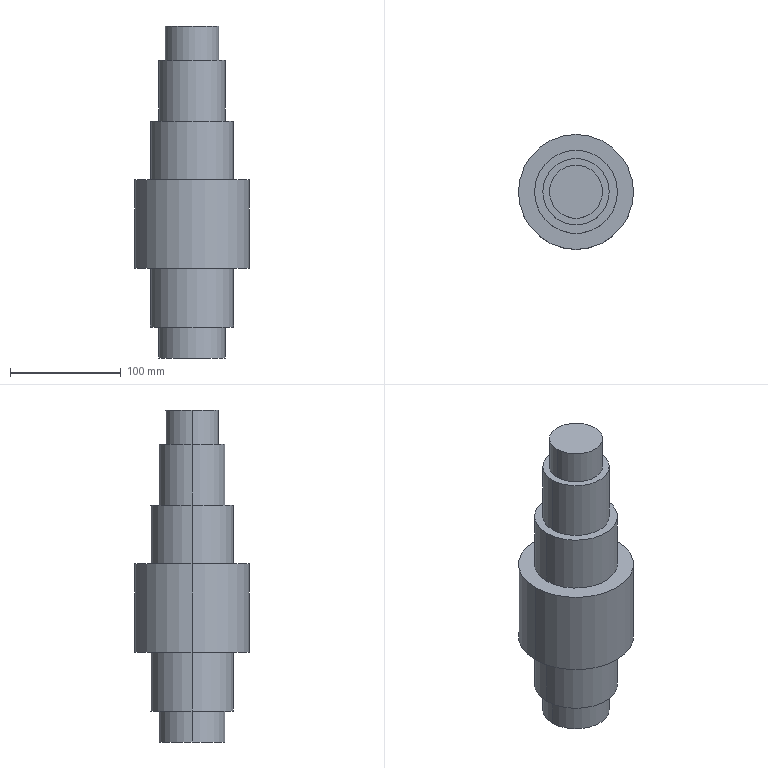Part | SolidWorks | features ICE 5, Extrusion 1 | 1 solid | 19 faces | box 103.893 x 103.893 x 300 mm | volume 1437259 mm3 | cylinder 12 | plane 7 | commonest cylinder face diameters 60 x4 75 x4 48 x2 103.893 x2
STEP:
#1=CARTESIAN_POINT('',(24.,0.,300.));
#2=VERTEX_POINT('',#1);
#3=CARTESIAN_POINT('',(-24.,0.,300.));
#4=VERTEX_POINT('',#3);
#5=CARTESIAN_POINT('',(0.,0.,300.));
#6=DIRECTION('',(0.,0.,1.));
#7=DIRECTION('',(1.,0.,0.));
#8=AXIS2_PLACEMENT_3D('',#5,#6,#7);
#9=CIRCLE('',#8,24.);
#10=EDGE_CURVE('',#2,#4,#9,.T.);
#11=ORIENTED_EDGE('',*,*,#10,.F.);
#12=CARTESIAN_POINT('',(24.,0.,269.));
#13=VERTEX_POINT('',#12);
#14=CARTESIAN_POINT('',(24.,0.,300.));
#15=DIRECTION('',(0.,0.,-1.));
#16=VECTOR('',#15,1000.);
#17=LINE('',#14,#16);
#18=EDGE_CURVE('',#2,#13,#17,.T.);
#19=ORIENTED_EDGE('',*,*,#18,.T.);
#20=CARTESIAN_POINT('',(-24.,0.,269.));
#21=VERTEX_POINT('',#20);
#22=CARTESIAN_POINT('',(0.,0.,269.));
#23=DIRECTION('',(0.,0.,1.));
#24=DIRECTION('',(1.,0.,0.));
#25=AXIS2_PLACEMENT_3D('',#22,#23,#24);
#26=CIRCLE('',#25,24.);
#27=EDGE_CURVE('',#13,#21,#26,.T.);
#28=ORIENTED_EDGE('',*,*,#27,.T.);
#29=CARTESIAN_POINT('',(-24.,0.,300.));
#30=DIRECTION('',(0.,0.,-1.));
#31=VECTOR('',#30,1000.);
#32=LINE('',#29,#31);
#33=EDGE_CURVE('',#4,#21,#32,.T.);
#34=ORIENTED_EDGE('',*,*,#33,.F.);
#35=EDGE_LOOP('',(#11,#19,#28,#34));
#36=FACE_OUTER_BOUND('',#35,.T.);
#37=CARTESIAN_POINT('',(0.,0.,300.));
#38=DIRECTION('',(0.,0.,-1.));
#39=DIRECTION('',(-1.,0.,0.));
#40=AXIS2_PLACEMENT_3D('',#37,#38,#39);
#41=CYLINDRICAL_SURFACE('',#40,24.);
#42=ADVANCED_FACE('',(#36),#41,.T.);
#43=CARTESIAN_POINT('',(30.,0.,269.));
#44=VERTEX_POINT('',#43);
#45=CARTESIAN_POINT('',(-30.,0.,269.));
#46=VERTEX_POINT('',#45);
#47=CARTESIAN_POINT('',(0.,0.,269.));
#48=DIRECTION('',(0.,0.,1.));
#49=DIRECTION('',(1.,0.,0.));
#50=AXIS2_PLACEMENT_3D('',#47,#48,#49);
#51=CIRCLE('',#50,30.);
#52=EDGE_CURVE('',#44,#46,#51,.T.);
#53=ORIENTED_EDGE('',*,*,#52,.F.);
#54=CARTESIAN_POINT('',(30.,0.,214.));
#55=VERTEX_POINT('',#54);
#56=CARTESIAN_POINT('',(30.,0.,269.));
#57=DIRECTION('',(0.,0.,-1.));
#58=VECTOR('',#57,1000.);
#59=LINE('',#56,#58);
#60=EDGE_CURVE('',#44,#55,#59,.T.);
#61=ORIENTED_EDGE('',*,*,#60,.T.);
#62=CARTESIAN_POINT('',(-30.,0.,214.));
#63=VERTEX_POINT('',#62);
#64=CARTESIAN_POINT('',(0.,0.,214.));
#65=DIRECTION('',(0.,0.,1.));
#66=DIRECTION('',(1.,0.,0.));
#67=AXIS2_PLACEMENT_3D('',#64,#65,#66);
#68=CIRCLE('',#67,30.);
#69=EDGE_CURVE('',#55,#63,#68,.T.);
#70=ORIENTED_EDGE('',*,*,#69,.T.);
#71=CARTESIAN_POINT('',(-30.,0.,269.));
#72=DIRECTION('',(0.,0.,-1.));
#73=VECTOR('',#72,1000.);
#74=LINE('',#71,#73);
#75=EDGE_CURVE('',#46,#63,#74,.T.);
#76=ORIENTED_EDGE('',*,*,#75,.F.);
#77=EDGE_LOOP('',(#53,#61,#70,#76));
#78=FACE_OUTER_BOUND('',#77,.T.);
#79=CARTESIAN_POINT('',(0.,0.,269.));
#80=DIRECTION('',(0.,0.,-1.));
#81=DIRECTION('',(-1.,0.,0.));
#82=AXIS2_PLACEMENT_3D('',#79,#80,#81);
#83=CYLINDRICAL_SURFACE('',#82,30.);
#84=ADVANCED_FACE('',(#78),#83,.T.);
#85=CARTESIAN_POINT('',(37.5,0.,214.));
#86=VERTEX_POINT('',#85);
#87=CARTESIAN_POINT('',(-37.5,0.,214.));
#88=VERTEX_POINT('',#87);
#89=CARTESIAN_POINT('',(0.,0.,214.));
#90=DIRECTION('',(0.,0.,1.));
#91=DIRECTION('',(1.,0.,0.));
#92=AXIS2_PLACEMENT_3D('',#89,#90,#91);
#93=CIRCLE('',#92,37.5);
#94=EDGE_CURVE('',#86,#88,#93,.T.);
#95=ORIENTED_EDGE('',*,*,#94,.F.);
#96=CARTESIAN_POINT('',(37.5,0.,161.));
#97=VERTEX_POINT('',#96);
#98=CARTESIAN_POINT('',(37.5,0.,214.));
#99=DIRECTION('',(0.,0.,-1.));
#100=VECTOR('',#99,1000.);
#101=LINE('',#98,#100);
#102=EDGE_CURVE('',#86,#97,#101,.T.);
#103=ORIENTED_EDGE('',*,*,#102,.T.);
#104=CARTESIAN_POINT('',(-37.5,0.,161.));
#105=VERTEX_POINT('',#104);
#106=CARTESIAN_POINT('',(0.,0.,161.));
#107=DIRECTION('',(0.,0.,1.));
#108=DIRECTION('',(1.,0.,0.));
#109=AXIS2_PLACEMENT_3D('',#106,#107,#108);
#110=CIRCLE('',#109,37.5);
#111=EDGE_CURVE('',#97,#105,#110,.T.);
#112=ORIENTED_EDGE('',*,*,#111,.T.);
#113=CARTESIAN_POINT('',(-37.5,0.,214.));
#114=DIRECTION('',(0.,0.,-1.));
#115=VECTOR('',#114,1000.);
#116=LINE('',#113,#115);
#117=EDGE_CURVE('',#88,#105,#116,.T.);
#118=ORIENTED_EDGE('',*,*,#117,.F.);
#119=EDGE_LOOP('',(#95,#103,#112,#118));
#120=FACE_OUTER_BOUND('',#119,.T.);
#121=CARTESIAN_POINT('',(0.,0.,214.));
#122=DIRECTION('',(0.,0.,-1.));
#123=DIRECTION('',(-1.,0.,0.));
#124=AXIS2_PLACEMENT_3D('',#121,#122,#123);
#125=CYLINDRICAL_SURFACE('',#124,37.5);
#126=ADVANCED_FACE('',(#120),#125,.T.);
#127=CARTESIAN_POINT('',(51.947,0.,161.));
#128=VERTEX_POINT('',#127);
#129=CARTESIAN_POINT('',(-51.947,0.,161.));
#130=VERTEX_POINT('',#129);
#131=CARTESIAN_POINT('',(0.,0.,161.));
#132=DIRECTION('',(0.,0.,1.));
#133=DIRECTION('',(1.,0.,0.));
#134=AXIS2_PLACEMENT_3D('',#131,#132,#133);
#135=CIRCLE('',#134,51.947);
#136=EDGE_CURVE('',#128,#130,#135,.T.);
#137=ORIENTED_EDGE('',*,*,#136,.F.);
#138=CARTESIAN_POINT('',(51.947,0.,81.));
#139=VERTEX_POINT('',#138);
#140=CARTESIAN_POINT('',(51.947,0.,161.));
#141=DIRECTION('',(0.,0.,-1.));
#142=VECTOR('',#141,1000.);
#143=LINE('',#140,#142);
#144=EDGE_CURVE('',#128,#139,#143,.T.);
#145=ORIENTED_EDGE('',*,*,#144,.T.);
#146=CARTESIAN_POINT('',(-51.947,0.,81.));
#147=VERTEX_POINT('',#146);
#148=CARTESIAN_POINT('',(0.,0.,81.));
#149=DIRECTION('',(0.,0.,1.));
#150=DIRECTION('',(1.,0.,0.));
#151=AXIS2_PLACEMENT_3D('',#148,#149,#150);
#152=CIRCLE('',#151,51.947);
#153=EDGE_CURVE('',#139,#147,#152,.T.);
#154=ORIENTED_EDGE('',*,*,#153,.T.);
#155=CARTESIAN_POINT('',(-51.947,0.,161.));
#156=DIRECTION('',(0.,0.,-1.));
#157=VECTOR('',#156,1000.);
#158=LINE('',#155,#157);
#159=EDGE_CURVE('',#130,#147,#158,.T.);
#160=ORIENTED_EDGE('',*,*,#159,.F.);
#161=EDGE_LOOP('',(#137,#145,#154,#160));
#162=FACE_OUTER_BOUND('',#161,.T.);
#163=CARTESIAN_POINT('',(0.,0.,161.));
#164=DIRECTION('',(0.,0.,-1.));
#165=DIRECTION('',(-1.,0.,0.));
#166=AXIS2_PLACEMENT_3D('',#163,#164,#165);
#167=CYLINDRICAL_SURFACE('',#166,51.947);
#168=ADVANCED_FACE('',(#162),#167,.T.);
#169=CARTESIAN_POINT('',(37.5,0.,81.));
#170=VERTEX_POINT('',#169);
#171=CARTESIAN_POINT('',(-37.5,0.,81.));
#172=VERTEX_POINT('',#171);
#173=CARTESIAN_POINT('',(0.,0.,81.));
#174=DIRECTION('',(0.,0.,1.));
#175=DIRECTION('',(1.,0.,0.));
#176=AXIS2_PLACEMENT_3D('',#173,#174,#175);
#177=CIRCLE('',#176,37.5);
#178=EDGE_CURVE('',#170,#172,#177,.T.);
#179=ORIENTED_EDGE('',*,*,#178,.F.);
#180=CARTESIAN_POINT('',(37.5,0.,28.));
#181=VERTEX_POINT('',#180);
#182=CARTESIAN_POINT('',(37.5,0.,81.));
#183=DIRECTION('',(0.,0.,-1.));
#184=VECTOR('',#183,1000.);
#185=LINE('',#182,#184);
#186=EDGE_CURVE('',#170,#181,#185,.T.);
#187=ORIENTED_EDGE('',*,*,#186,.T.);
#188=CARTESIAN_POINT('',(-37.5,0.,28.));
#189=VERTEX_POINT('',#188);
#190=CARTESIAN_POINT('',(0.,0.,28.));
#191=DIRECTION('',(0.,0.,1.));
#192=DIRECTION('',(1.,0.,0.));
#193=AXIS2_PLACEMENT_3D('',#190,#191,#192);
#194=CIRCLE('',#193,37.5);
#195=EDGE_CURVE('',#181,#189,#194,.T.);
#196=ORIENTED_EDGE('',*,*,#195,.T.);
#197=CARTESIAN_POINT('',(-37.5,0.,81.));
#198=DIRECTION('',(0.,0.,-1.));
#199=VECTOR('',#198,1000.);
#200=LINE('',#197,#199);
#201=EDGE_CURVE('',#172,#189,#200,.T.);
#202=ORIENTED_EDGE('',*,*,#201,.F.);
#203=EDGE_LOOP('',(#179,#187,#196,#202));
#204=FACE_OUTER_BOUND('',#203,.T.);
#205=CARTESIAN_POINT('',(0.,0.,81.));
#206=DIRECTION('',(0.,0.,-1.));
#207=DIRECTION('',(-1.,0.,0.));
#208=AXIS2_PLACEMENT_3D('',#205,#206,#207);
#209=CYLINDRICAL_SURFACE('',#208,37.5);
#210=ADVANCED_FACE('',(#204),#209,.T.);
#211=CARTESIAN_POINT('',(30.,0.,28.));
#212=VERTEX_POINT('',#211);
#213=CARTESIAN_POINT('',(-30.,0.,28.));
#214=VERTEX_POINT('',#213);
#215=CARTESIAN_POINT('',(0.,0.,28.));
#216=DIRECTION('',(0.,0.,1.));
#217=DIRECTION('',(1.,0.,0.));
#218=AXIS2_PLACEMENT_3D('',#215,#216,#217);
#219=CIRCLE('',#218,30.);
#220=EDGE_CURVE('',#212,#214,#219,.T.);
#221=ORIENTED_EDGE('',*,*,#220,.F.);
#222=CARTESIAN_POINT('',(30.,0.,0.));
#223=VERTEX_POINT('',#222);
#224=CARTESIAN_POINT('',(30.,0.,28.));
#225=DIRECTION('',(0.,0.,-1.));
#226=VECTOR('',#225,1000.);
#227=LINE('',#224,#226);
#228=EDGE_CURVE('',#212,#223,#227,.T.);
#229=ORIENTED_EDGE('',*,*,#228,.T.);
#230=CARTESIAN_POINT('',(-30.,0.,0.));
#231=VERTEX_POINT('',#230);
#232=CARTESIAN_POINT('',(0.,0.,0.));
#233=DIRECTION('',(0.,0.,1.));
#234=DIRECTION('',(1.,0.,0.));
#235=AXIS2_PLACEMENT_3D('',#232,#233,#234);
#236=CIRCLE('',#235,30.);
#237=EDGE_CURVE('',#223,#231,#236,.T.);
#238=ORIENTED_EDGE('',*,*,#237,.T.);
#239=CARTESIAN_POINT('',(-30.,0.,28.));
#240=DIRECTION('',(0.,0.,-1.));
#241=VECTOR('',#240,1000.);
#242=LINE('',#239,#241);
#243=EDGE_CURVE('',#214,#231,#242,.T.);
#244=ORIENTED_EDGE('',*,*,#243,.F.);
#245=EDGE_LOOP('',(#221,#229,#238,#244));
#246=FACE_OUTER_BOUND('',#245,.T.);
#247=CARTESIAN_POINT('',(0.,0.,28.));
#248=DIRECTION('',(0.,0.,-1.));
#249=DIRECTION('',(-1.,0.,0.));
#250=AXIS2_PLACEMENT_3D('',#247,#248,#249);
#251=CYLINDRICAL_SURFACE('',#250,30.);
#252=ADVANCED_FACE('',(#246),#251,.T.);
#253=CARTESIAN_POINT('',(0.,0.,269.));
#254=DIRECTION('',(0.,0.,1.));
#255=DIRECTION('',(1.,0.,0.));
#256=AXIS2_PLACEMENT_3D('',#253,#254,#255);
#257=CIRCLE('',#256,30.);
#258=EDGE_CURVE('',#46,#44,#257,.T.);
#259=ORIENTED_EDGE('',*,*,#258,.T.);
#260=ORIENTED_EDGE('',*,*,#52,.T.);
#261=EDGE_LOOP('',(#259,#260));
#262=FACE_OUTER_BOUND('',#261,.T.);
#263=CARTESIAN_POINT('',(0.,0.,269.));
#264=DIRECTION('',(0.,0.,1.));
#265=DIRECTION('',(1.,0.,0.));
#266=AXIS2_PLACEMENT_3D('',#263,#264,#265);
#267=CIRCLE('',#266,24.);
#268=EDGE_CURVE('',#21,#13,#267,.T.);
#269=ORIENTED_EDGE('',*,*,#268,.F.);
#270=ORIENTED_EDGE('',*,*,#27,.F.);
#271=EDGE_LOOP('',(#269,#270));
#272=FACE_BOUND('',#271,.T.);
#273=CARTESIAN_POINT('',(0.,0.,269.));
#274=DIRECTION('',(0.,0.,1.));
#275=DIRECTION('',(1.,0.,0.));
#276=AXIS2_PLACEMENT_3D('',#273,#274,#275);
#277=PLANE('',#276);
#278=ADVANCED_FACE('',(#262,#272),#277,.T.);
#279=CARTESIAN_POINT('',(0.,0.,214.));
#280=DIRECTION('',(0.,0.,1.));
#281=DIRECTION('',(1.,0.,0.));
#282=AXIS2_PLACEMENT_3D('',#279,#280,#281);
#283=CIRCLE('',#282,37.5);
#284=EDGE_CURVE('',#88,#86,#283,.T.);
#285=ORIENTED_EDGE('',*,*,#284,.T.);
#286=ORIENTED_EDGE('',*,*,#94,.T.);
#287=EDGE_LOOP('',(#285,#286));
#288=FACE_OUTER_BOUND('',#287,.T.);
#289=CARTESIAN_POINT('',(0.,0.,214.));
#290=DIRECTION('',(0.,0.,1.));
#291=DIRECTION('',(1.,0.,0.));
#292=AXIS2_PLACEMENT_3D('',#289,#290,#291);
#293=CIRCLE('',#292,30.);
#294=EDGE_CURVE('',#63,#55,#293,.T.);
#295=ORIENTED_EDGE('',*,*,#294,.F.);
#296=ORIENTED_EDGE('',*,*,#69,.F.);
#297=EDGE_LOOP('',(#295,#296));
#298=FACE_BOUND('',#297,.T.);
#299=CARTESIAN_POINT('',(0.,0.,214.));
#300=DIRECTION('',(0.,0.,1.));
#301=DIRECTION('',(1.,0.,0.));
#302=AXIS2_PLACEMENT_3D('',#299,#300,#301);
#303=PLANE('',#302);
#304=ADVANCED_FACE('',(#288,#298),#303,.T.);
#305=CARTESIAN_POINT('',(0.,0.,161.));
#306=DIRECTION('',(0.,0.,1.));
#307=DIRECTION('',(1.,0.,0.));
#308=AXIS2_PLACEMENT_3D('',#305,#306,#307);
#309=CIRCLE('',#308,51.947);
#310=EDGE_CURVE('',#130,#128,#309,.T.);
#311=ORIENTED_EDGE('',*,*,#310,.T.);
#312=ORIENTED_EDGE('',*,*,#136,.T.);
#313=EDGE_LOOP('',(#311,#312));
#314=FACE_OUTER_BOUND('',#313,.T.);
#315=CARTESIAN_POINT('',(0.,0.,161.));
#316=DIRECTION('',(0.,0.,1.));
#317=DIRECTION('',(1.,0.,0.));
#318=AXIS2_PLACEMENT_3D('',#315,#316,#317);
#319=CIRCLE('',#318,37.5);
#320=EDGE_CURVE('',#105,#97,#319,.T.);
#321=ORIENTED_EDGE('',*,*,#320,.F.);
#322=ORIENTED_EDGE('',*,*,#111,.F.);
#323=EDGE_LOOP('',(#321,#322));
#324=FACE_BOUND('',#323,.T.);
#325=CARTESIAN_POINT('',(0.,0.,161.));
#326=DIRECTION('',(0.,0.,1.));
#327=DIRECTION('',(1.,0.,0.));
#328=AXIS2_PLACEMENT_3D('',#325,#326,#327);
#329=PLANE('',#328);
#330=ADVANCED_FACE('',(#314,#324),#329,.T.);
#331=ORIENTED_EDGE('',*,*,#228,.F.);
#332=CARTESIAN_POINT('',(0.,0.,28.));
#333=DIRECTION('',(0.,0.,1.));
#334=DIRECTION('',(1.,0.,0.));
#335=AXIS2_PLACEMENT_3D('',#332,#333,#334);
#336=CIRCLE('',#335,30.);
#337=EDGE_CURVE('',#214,#212,#336,.T.);
#338=ORIENTED_EDGE('',*,*,#337,.F.);
#339=ORIENTED_EDGE('',*,*,#243,.T.);
#340=CARTESIAN_POINT('',(0.,0.,0.));
#341=DIRECTION('',(0.,0.,1.));
#342=DIRECTION('',(1.,0.,0.));
#343=AXIS2_PLACEMENT_3D('',#340,#341,#342);
#344=CIRCLE('',#343,30.);
#345=EDGE_CURVE('',#231,#223,#344,.T.);
#346=ORIENTED_EDGE('',*,*,#345,.T.);
#347=EDGE_LOOP('',(#331,#338,#339,#346));
#348=FACE_OUTER_BOUND('',#347,.T.);
#349=CARTESIAN_POINT('',(0.,0.,28.));
#350=DIRECTION('',(0.,0.,-1.));
#351=DIRECTION('',(-1.,0.,0.));
#352=AXIS2_PLACEMENT_3D('',#349,#350,#351);
#353=CYLINDRICAL_SURFACE('',#352,30.);
#354=ADVANCED_FACE('',(#348),#353,.T.);
#355=ORIENTED_EDGE('',*,*,#345,.F.);
#356=ORIENTED_EDGE('',*,*,#237,.F.);
#357=EDGE_LOOP('',(#355,#356));
#358=FACE_OUTER_BOUND('',#357,.T.);
#359=CARTESIAN_POINT('',(0.,0.,0.));
#360=DIRECTION('',(0.,0.,1.));
#361=DIRECTION('',(1.,0.,0.));
#362=AXIS2_PLACEMENT_3D('',#359,#360,#361);
#363=PLANE('',#362);
#364=ADVANCED_FACE('',(#358),#363,.F.);
#365=CARTESIAN_POINT('',(0.,0.,28.));
#366=DIRECTION('',(0.,0.,1.));
#367=DIRECTION('',(1.,0.,0.));
#368=AXIS2_PLACEMENT_3D('',#365,#366,#367);
#369=CIRCLE('',#368,37.5);
#370=EDGE_CURVE('',#189,#181,#369,.T.);
#371=ORIENTED_EDGE('',*,*,#370,.F.);
#372=ORIENTED_EDGE('',*,*,#195,.F.);
#373=EDGE_LOOP('',(#371,#372));
#374=FACE_OUTER_BOUND('',#373,.T.);
#375=ORIENTED_EDGE('',*,*,#337,.T.);
#376=ORIENTED_EDGE('',*,*,#220,.T.);
#377=EDGE_LOOP('',(#375,#376));
#378=FACE_BOUND('',#377,.T.);
#379=CARTESIAN_POINT('',(0.,0.,28.));
#380=DIRECTION('',(0.,0.,1.));
#381=DIRECTION('',(1.,0.,0.));
#382=AXIS2_PLACEMENT_3D('',#379,#380,#381);
#383=PLANE('',#382);
#384=ADVANCED_FACE('',(#374,#378),#383,.F.);
#385=ORIENTED_EDGE('',*,*,#186,.F.);
#386=CARTESIAN_POINT('',(0.,0.,81.));
#387=DIRECTION('',(0.,0.,1.));
#388=DIRECTION('',(1.,0.,0.));
#389=AXIS2_PLACEMENT_3D('',#386,#387,#388);
#390=CIRCLE('',#389,37.5);
#391=EDGE_CURVE('',#172,#170,#390,.T.);
#392=ORIENTED_EDGE('',*,*,#391,.F.);
#393=ORIENTED_EDGE('',*,*,#201,.T.);
#394=ORIENTED_EDGE('',*,*,#370,.T.);
#395=EDGE_LOOP('',(#385,#392,#393,#394));
#396=FACE_OUTER_BOUND('',#395,.T.);
#397=CARTESIAN_POINT('',(0.,0.,81.));
#398=DIRECTION('',(0.,0.,-1.));
#399=DIRECTION('',(-1.,0.,0.));
#400=AXIS2_PLACEMENT_3D('',#397,#398,#399);
#401=CYLINDRICAL_SURFACE('',#400,37.5);
#402=ADVANCED_FACE('',(#396),#401,.T.);
#403=CARTESIAN_POINT('',(0.,0.,81.));
#404=DIRECTION('',(0.,0.,1.));
#405=DIRECTION('',(1.,0.,0.));
#406=AXIS2_PLACEMENT_3D('',#403,#404,#405);
#407=CIRCLE('',#406,51.947);
#408=EDGE_CURVE('',#147,#139,#407,.T.);
#409=ORIENTED_EDGE('',*,*,#408,.F.);
#410=ORIENTED_EDGE('',*,*,#153,.F.);
#411=EDGE_LOOP('',(#409,#410));
#412=FACE_OUTER_BOUND('',#411,.T.);
#413=ORIENTED_EDGE('',*,*,#391,.T.);
#414=ORIENTED_EDGE('',*,*,#178,.T.);
#415=EDGE_LOOP('',(#413,#414));
#416=FACE_BOUND('',#415,.T.);
#417=CARTESIAN_POINT('',(0.,0.,81.));
#418=DIRECTION('',(0.,0.,1.));
#419=DIRECTION('',(1.,0.,0.));
#420=AXIS2_PLACEMENT_3D('',#417,#418,#419);
#421=PLANE('',#420);
#422=ADVANCED_FACE('',(#412,#416),#421,.F.);
#423=ORIENTED_EDGE('',*,*,#144,.F.);
#424=ORIENTED_EDGE('',*,*,#310,.F.);
#425=ORIENTED_EDGE('',*,*,#159,.T.);
#426=ORIENTED_EDGE('',*,*,#408,.T.);
#427=EDGE_LOOP('',(#423,#424,#425,#426));
#428=FACE_OUTER_BOUND('',#427,.T.);
#429=CARTESIAN_POINT('',(0.,0.,161.));
#430=DIRECTION('',(0.,0.,-1.));
#431=DIRECTION('',(-1.,0.,0.));
#432=AXIS2_PLACEMENT_3D('',#429,#430,#431);
#433=CYLINDRICAL_SURFACE('',#432,51.947);
#434=ADVANCED_FACE('',(#428),#433,.T.);
#435=ORIENTED_EDGE('',*,*,#102,.F.);
#436=ORIENTED_EDGE('',*,*,#284,.F.);
#437=ORIENTED_EDGE('',*,*,#117,.T.);
#438=ORIENTED_EDGE('',*,*,#320,.T.);
#439=EDGE_LOOP('',(#435,#436,#437,#438));
#440=FACE_OUTER_BOUND('',#439,.T.);
#441=CARTESIAN_POINT('',(0.,0.,214.));
#442=DIRECTION('',(0.,0.,-1.));
#443=DIRECTION('',(-1.,0.,0.));
#444=AXIS2_PLACEMENT_3D('',#441,#442,#443);
#445=CYLINDRICAL_SURFACE('',#444,37.5);
#446=ADVANCED_FACE('',(#440),#445,.T.);
#447=ORIENTED_EDGE('',*,*,#60,.F.);
#448=ORIENTED_EDGE('',*,*,#258,.F.);
#449=ORIENTED_EDGE('',*,*,#75,.T.);
#450=ORIENTED_EDGE('',*,*,#294,.T.);
#451=EDGE_LOOP('',(#447,#448,#449,#450));
#452=FACE_OUTER_BOUND('',#451,.T.);
#453=CARTESIAN_POINT('',(0.,0.,269.));
#454=DIRECTION('',(0.,0.,-1.));
#455=DIRECTION('',(-1.,0.,0.));
#456=AXIS2_PLACEMENT_3D('',#453,#454,#455);
#457=CYLINDRICAL_SURFACE('',#456,30.);
#458=ADVANCED_FACE('',(#452),#457,.T.);
#459=ORIENTED_EDGE('',*,*,#18,.F.);
#460=CARTESIAN_POINT('',(0.,0.,300.));
#461=DIRECTION('',(0.,0.,1.));
#462=DIRECTION('',(1.,0.,0.));
#463=AXIS2_PLACEMENT_3D('',#460,#461,#462);
#464=CIRCLE('',#463,24.);
#465=EDGE_CURVE('',#4,#2,#464,.T.);
#466=ORIENTED_EDGE('',*,*,#465,.F.);
#467=ORIENTED_EDGE('',*,*,#33,.T.);
#468=ORIENTED_EDGE('',*,*,#268,.T.);
#469=EDGE_LOOP('',(#459,#466,#467,#468));
#470=FACE_OUTER_BOUND('',#469,.T.);
#471=CARTESIAN_POINT('',(0.,0.,300.));
#472=DIRECTION('',(0.,0.,-1.));
#473=DIRECTION('',(-1.,0.,0.));
#474=AXIS2_PLACEMENT_3D('',#471,#472,#473);
#475=CYLINDRICAL_SURFACE('',#474,24.);
#476=ADVANCED_FACE('',(#470),#475,.T.);
#477=ORIENTED_EDGE('',*,*,#465,.T.);
#478=ORIENTED_EDGE('',*,*,#10,.T.);
#479=EDGE_LOOP('',(#477,#478));
#480=FACE_OUTER_BOUND('',#479,.T.);
#481=CARTESIAN_POINT('',(0.,0.,300.));
#482=DIRECTION('',(0.,0.,1.));
#483=DIRECTION('',(1.,0.,0.));
#484=AXIS2_PLACEMENT_3D('',#481,#482,#483);
#485=PLANE('',#484);
#486=ADVANCED_FACE('',(#480),#485,.T.);
#487=CLOSED_SHELL('',(#42,#84,#126,#168,#210,#252,#278,#304,#330,#354,#364,#384,#402,#422,#434,#446,#458,#476,#486));
#488=MANIFOLD_SOLID_BREP('',#487);
#489=CARTESIAN_POINT('',(0.,0.,0.));
#490=DIRECTION('',(0.,0.,1.));
#491=DIRECTION('',(1.,0.,0.));
#492=AXIS2_PLACEMENT_3D('',#489,#490,#491);
#493=(LENGTH_UNIT()NAMED_UNIT(*)SI_UNIT(.MILLI.,.METRE.));
#494=UNCERTAINTY_MEASURE_WITH_UNIT(LENGTH_MEASURE(0.00001),#493,'','');
#495=(NAMED_UNIT(*)PLANE_ANGLE_UNIT()SI_UNIT($,.RADIAN.));
#496=(NAMED_UNIT(*)SI_UNIT($,.STERADIAN.)SOLID_ANGLE_UNIT());
#497=(GEOMETRIC_REPRESENTATION_CONTEXT(3)GLOBAL_UNCERTAINTY_ASSIGNED_CONTEXT((#494))GLOBAL_UNIT_ASSIGNED_CONTEXT((#493,#495,#496))REPRESENTATION_CONTEXT('',''));
#498=ADVANCED_BREP_SHAPE_REPRESENTATION('',(#488,#492),#497);